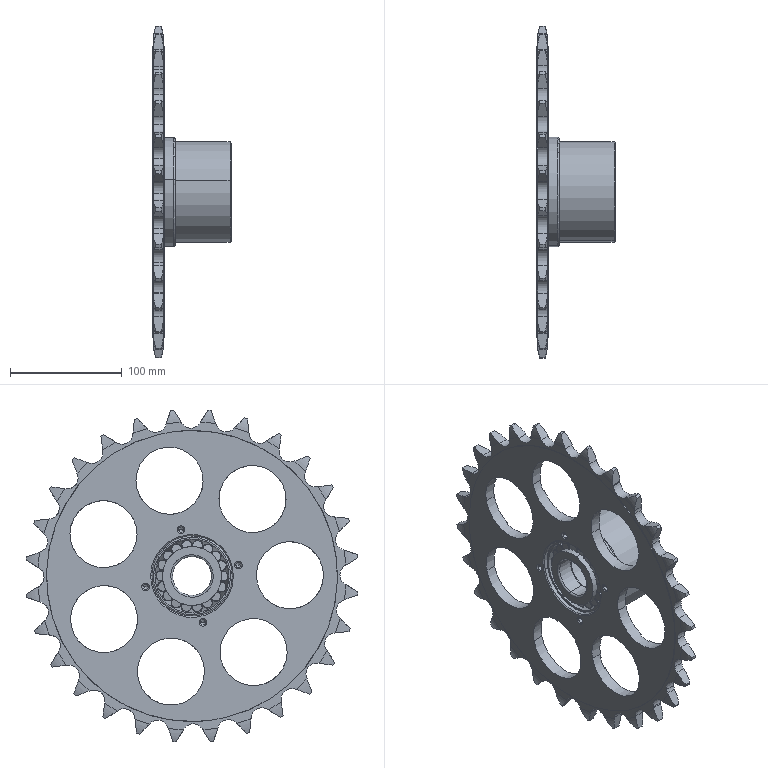Part | STEP file | Drive sprocket | 1 solid | 687 faces | box 70 x 296.646 x 296.646 mm | volume 579512 mm3 | torus 290 | plane 151 | cylinder 138 | cone 108 | commonest cylinder face diameters 19.25 x46 298 x28 60 x14 5 x8 165 x7 185 x7